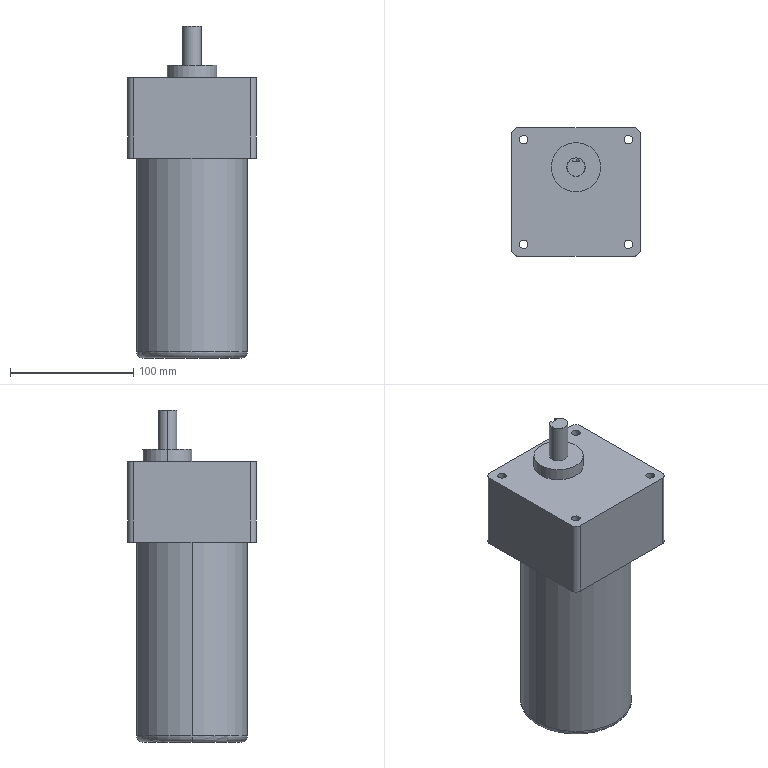Part | STEP file | Taibang reversible motor 90W_Default | 1 solid | 37 faces | box 104 x 104 x 269 mm | volume 1739193 mm3 | cylinder 20 | plane 12 | cone 3 | torus 2 | commonest cylinder face diameters 6.8 x8 10 x4 5 x2 15 x2 40 x2 90 x2